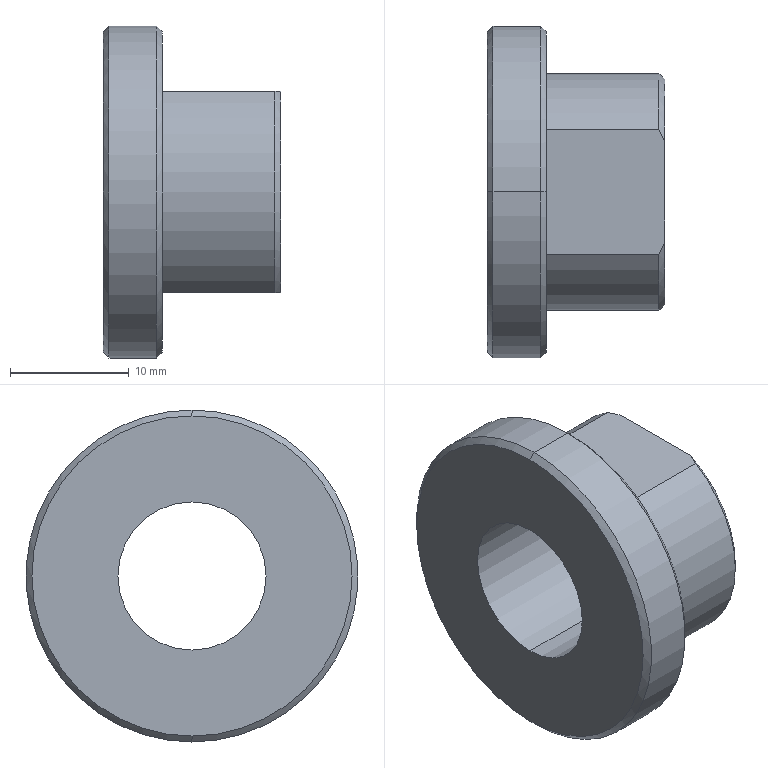Part | SolidWorks | features BaseBody 1 | 1 solid | 17 faces | box 15 x 28 x 28 mm | volume 4139 mm3 | cylinder 6 | cone 6 | plane 5 | commonest cylinder face diameters 12.5 x2 20 x2 28 x2
STEP:
#1=CARTESIAN_POINT('',(0.,0.,6.25));
#2=VERTEX_POINT('',#1);
#3=CARTESIAN_POINT('',(0.,0.,-6.25));
#4=VERTEX_POINT('',#3);
#5=CARTESIAN_POINT('',(0.,0.,0.));
#6=DIRECTION('',(1.,0.,0.));
#7=DIRECTION('',(0.,0.,-1.));
#8=AXIS2_PLACEMENT_3D('',#5,#6,#7);
#9=CIRCLE('',#8,6.25);
#10=EDGE_CURVE('',#2,#4,#9,.T.);
#11=ORIENTED_EDGE('',*,*,#10,.F.);
#12=CARTESIAN_POINT('',(15.,0.,6.25));
#13=VERTEX_POINT('',#12);
#14=CARTESIAN_POINT('',(15.,0.,6.25));
#15=DIRECTION('',(1.,0.,0.));
#16=VECTOR('',#15,1000.);
#17=LINE('',#14,#16);
#18=EDGE_CURVE('',#2,#13,#17,.T.);
#19=ORIENTED_EDGE('',*,*,#18,.T.);
#20=CARTESIAN_POINT('',(15.,0.,-6.25));
#21=VERTEX_POINT('',#20);
#22=CARTESIAN_POINT('',(15.,0.,0.));
#23=DIRECTION('',(1.,0.,0.));
#24=DIRECTION('',(0.,0.,-1.));
#25=AXIS2_PLACEMENT_3D('',#22,#23,#24);
#26=CIRCLE('',#25,6.25);
#27=EDGE_CURVE('',#13,#21,#26,.T.);
#28=ORIENTED_EDGE('',*,*,#27,.T.);
#29=CARTESIAN_POINT('',(15.,0.,-6.25));
#30=DIRECTION('',(1.,0.,0.));
#31=VECTOR('',#30,1000.);
#32=LINE('',#29,#31);
#33=EDGE_CURVE('',#4,#21,#32,.T.);
#34=ORIENTED_EDGE('',*,*,#33,.F.);
#35=EDGE_LOOP('',(#11,#19,#28,#34));
#36=FACE_OUTER_BOUND('',#35,.T.);
#37=CARTESIAN_POINT('',(15.,0.,0.));
#38=DIRECTION('',(1.,0.,0.));
#39=DIRECTION('',(0.,0.,-1.));
#40=AXIS2_PLACEMENT_3D('',#37,#38,#39);
#41=CYLINDRICAL_SURFACE('',#40,6.25);
#42=ADVANCED_FACE('',(#36),#41,.F.);
#43=CARTESIAN_POINT('',(0.,0.,13.5));
#44=VERTEX_POINT('',#43);
#45=CARTESIAN_POINT('',(0.,0.,-13.5));
#46=VERTEX_POINT('',#45);
#47=CARTESIAN_POINT('',(0.,0.,0.));
#48=DIRECTION('',(-1.,0.,0.));
#49=DIRECTION('',(0.,0.,-1.));
#50=AXIS2_PLACEMENT_3D('',#47,#48,#49);
#51=CIRCLE('',#50,13.5);
#52=EDGE_CURVE('',#44,#46,#51,.T.);
#53=ORIENTED_EDGE('',*,*,#52,.F.);
#54=CARTESIAN_POINT('',(0.5,0.,14.));
#55=VERTEX_POINT('',#54);
#56=CARTESIAN_POINT('',(0.5,0.,14.));
#57=DIRECTION('',(0.7071,0.,0.7071));
#58=VECTOR('',#57,1000.);
#59=LINE('',#56,#58);
#60=EDGE_CURVE('',#44,#55,#59,.T.);
#61=ORIENTED_EDGE('',*,*,#60,.T.);
#62=CARTESIAN_POINT('',(0.5,0.,-14.));
#63=VERTEX_POINT('',#62);
#64=CARTESIAN_POINT('',(0.5,0.,0.));
#65=DIRECTION('',(1.,0.,0.));
#66=DIRECTION('',(0.,0.,-1.));
#67=AXIS2_PLACEMENT_3D('',#64,#65,#66);
#68=CIRCLE('',#67,14.);
#69=EDGE_CURVE('',#63,#55,#68,.T.);
#70=ORIENTED_EDGE('',*,*,#69,.F.);
#71=CARTESIAN_POINT('',(0.5,0.,-14.));
#72=DIRECTION('',(0.7071,0.,-0.7071));
#73=VECTOR('',#72,1000.);
#74=LINE('',#71,#73);
#75=EDGE_CURVE('',#46,#63,#74,.T.);
#76=ORIENTED_EDGE('',*,*,#75,.F.);
#77=EDGE_LOOP('',(#53,#61,#70,#76));
#78=FACE_OUTER_BOUND('',#77,.T.);
#79=CARTESIAN_POINT('',(0.5,0.,0.));
#80=DIRECTION('',(1.,0.,0.));
#81=DIRECTION('',(0.,0.,-1.));
#82=AXIS2_PLACEMENT_3D('',#79,#80,#81);
#83=CONICAL_SURFACE('',#82,14.,0.7854);
#84=ADVANCED_FACE('',(#78),#83,.T.);
#85=CARTESIAN_POINT('',(5.,0.,-13.5));
#86=VERTEX_POINT('',#85);
#87=CARTESIAN_POINT('',(5.,0.,13.5));
#88=VERTEX_POINT('',#87);
#89=CARTESIAN_POINT('',(5.,0.,0.));
#90=DIRECTION('',(1.,0.,0.));
#91=DIRECTION('',(0.,0.,-1.));
#92=AXIS2_PLACEMENT_3D('',#89,#90,#91);
#93=CIRCLE('',#92,13.5);
#94=EDGE_CURVE('',#86,#88,#93,.T.);
#95=ORIENTED_EDGE('',*,*,#94,.F.);
#96=CARTESIAN_POINT('',(4.5,0.,-14.));
#97=VERTEX_POINT('',#96);
#98=CARTESIAN_POINT('',(5.,0.,-13.5));
#99=DIRECTION('',(-0.7071,0.,-0.7071));
#100=VECTOR('',#99,1000.);
#101=LINE('',#98,#100);
#102=EDGE_CURVE('',#86,#97,#101,.T.);
#103=ORIENTED_EDGE('',*,*,#102,.T.);
#104=CARTESIAN_POINT('',(4.5,0.,14.));
#105=VERTEX_POINT('',#104);
#106=CARTESIAN_POINT('',(4.5,0.,0.));
#107=DIRECTION('',(-1.,0.,0.));
#108=DIRECTION('',(0.,0.,-1.));
#109=AXIS2_PLACEMENT_3D('',#106,#107,#108);
#110=CIRCLE('',#109,14.);
#111=EDGE_CURVE('',#105,#97,#110,.T.);
#112=ORIENTED_EDGE('',*,*,#111,.F.);
#113=CARTESIAN_POINT('',(5.,0.,13.5));
#114=DIRECTION('',(-0.7071,0.,0.7071));
#115=VECTOR('',#114,1000.);
#116=LINE('',#113,#115);
#117=EDGE_CURVE('',#88,#105,#116,.T.);
#118=ORIENTED_EDGE('',*,*,#117,.F.);
#119=EDGE_LOOP('',(#95,#103,#112,#118));
#120=FACE_OUTER_BOUND('',#119,.T.);
#121=CARTESIAN_POINT('',(5.,0.,0.));
#122=DIRECTION('',(-1.,0.,0.));
#123=DIRECTION('',(0.,0.,1.));
#124=AXIS2_PLACEMENT_3D('',#121,#122,#123);
#125=CONICAL_SURFACE('',#124,13.5,0.7854);
#126=ADVANCED_FACE('',(#120),#125,.T.);
#127=ORIENTED_EDGE('',*,*,#111,.T.);
#128=CARTESIAN_POINT('',(5.,0.,-14.));
#129=DIRECTION('',(-1.,0.,0.));
#130=VECTOR('',#129,1000.);
#131=LINE('',#128,#130);
#132=EDGE_CURVE('',#97,#63,#131,.T.);
#133=ORIENTED_EDGE('',*,*,#132,.T.);
#134=ORIENTED_EDGE('',*,*,#69,.T.);
#135=CARTESIAN_POINT('',(5.,0.,14.));
#136=DIRECTION('',(-1.,0.,0.));
#137=VECTOR('',#136,1000.);
#138=LINE('',#135,#137);
#139=EDGE_CURVE('',#105,#55,#138,.T.);
#140=ORIENTED_EDGE('',*,*,#139,.F.);
#141=EDGE_LOOP('',(#127,#133,#134,#140));
#142=FACE_OUTER_BOUND('',#141,.T.);
#143=CARTESIAN_POINT('',(5.,0.,0.));
#144=DIRECTION('',(-1.,0.,0.));
#145=DIRECTION('',(0.,0.,1.));
#146=AXIS2_PLACEMENT_3D('',#143,#144,#145);
#147=CYLINDRICAL_SURFACE('',#146,14.);
#148=ADVANCED_FACE('',(#142),#147,.T.);
#149=CARTESIAN_POINT('',(14.5,-5.268,-8.5));
#150=VERTEX_POINT('',#149);
#151=CARTESIAN_POINT('',(14.5,-5.268,8.5));
#152=VERTEX_POINT('',#151);
#153=CARTESIAN_POINT('',(14.5,0.,0.));
#154=DIRECTION('',(-1.,0.,0.));
#155=DIRECTION('',(0.,0.,-1.));
#156=AXIS2_PLACEMENT_3D('',#153,#154,#155);
#157=CIRCLE('',#156,10.);
#158=EDGE_CURVE('',#150,#152,#157,.T.);
#159=ORIENTED_EDGE('',*,*,#158,.T.);
#160=CARTESIAN_POINT('',(5.,-5.268,8.5));
#161=VERTEX_POINT('',#160);
#162=CARTESIAN_POINT('',(15.,-5.268,8.5));
#163=DIRECTION('',(-1.,0.,0.));
#164=VECTOR('',#163,1000.);
#165=LINE('',#162,#164);
#166=EDGE_CURVE('',#152,#161,#165,.T.);
#167=ORIENTED_EDGE('',*,*,#166,.T.);
#168=CARTESIAN_POINT('',(5.,-5.268,-8.5));
#169=VERTEX_POINT('',#168);
#170=CARTESIAN_POINT('',(5.,0.,0.));
#171=DIRECTION('',(1.,0.,0.));
#172=DIRECTION('',(0.,0.,-1.));
#173=AXIS2_PLACEMENT_3D('',#170,#171,#172);
#174=CIRCLE('',#173,10.);
#175=EDGE_CURVE('',#161,#169,#174,.T.);
#176=ORIENTED_EDGE('',*,*,#175,.T.);
#177=CARTESIAN_POINT('',(15.,-5.268,-8.5));
#178=DIRECTION('',(1.,0.,0.));
#179=VECTOR('',#178,1000.);
#180=LINE('',#177,#179);
#181=EDGE_CURVE('',#169,#150,#180,.T.);
#182=ORIENTED_EDGE('',*,*,#181,.T.);
#183=EDGE_LOOP('',(#159,#167,#176,#182));
#184=FACE_OUTER_BOUND('',#183,.T.);
#185=CARTESIAN_POINT('',(15.,0.,0.));
#186=DIRECTION('',(-1.,0.,0.));
#187=DIRECTION('',(0.,0.,1.));
#188=AXIS2_PLACEMENT_3D('',#185,#186,#187);
#189=CYLINDRICAL_SURFACE('',#188,10.);
#190=ADVANCED_FACE('',(#184),#189,.T.);
#191=CARTESIAN_POINT('',(15.,-4.243,8.5));
#192=VERTEX_POINT('',#191);
#193=CARTESIAN_POINT('',(14.5,-5.268,8.5));
#194=CARTESIAN_POINT('',(14.677,-4.931,8.5));
#195=CARTESIAN_POINT('',(14.845,-4.59,8.5));
#196=CARTESIAN_POINT('',(15.,-4.243,8.5));
#197=B_SPLINE_CURVE_WITH_KNOTS('',3,(#193,#194,#195,#196),.UNSPECIFIED.,.F.,.F.,(4,4),(0.01928,0.02042),.UNSPECIFIED.);
#198=EDGE_CURVE('',#152,#192,#197,.T.);
#199=ORIENTED_EDGE('',*,*,#198,.F.);
#200=ORIENTED_EDGE('',*,*,#158,.F.);
#201=CARTESIAN_POINT('',(15.,-4.243,-8.5));
#202=VERTEX_POINT('',#201);
#203=CARTESIAN_POINT('',(15.,-4.243,-8.5));
#204=CARTESIAN_POINT('',(14.844,-4.591,-8.5));
#205=CARTESIAN_POINT('',(14.677,-4.932,-8.5));
#206=CARTESIAN_POINT('',(14.5,-5.268,-8.5));
#207=B_SPLINE_CURVE_WITH_KNOTS('',3,(#203,#204,#205,#206),.UNSPECIFIED.,.F.,.F.,(4,4),(0.02921,0.03036),.UNSPECIFIED.);
#208=EDGE_CURVE('',#202,#150,#207,.T.);
#209=ORIENTED_EDGE('',*,*,#208,.F.);
#210=CARTESIAN_POINT('',(15.,0.,0.));
#211=DIRECTION('',(1.,0.,0.));
#212=DIRECTION('',(0.,0.,-1.));
#213=AXIS2_PLACEMENT_3D('',#210,#211,#212);
#214=CIRCLE('',#213,9.5);
#215=EDGE_CURVE('',#192,#202,#214,.T.);
#216=ORIENTED_EDGE('',*,*,#215,.F.);
#217=EDGE_LOOP('',(#199,#200,#209,#216));
#218=FACE_OUTER_BOUND('',#217,.T.);
#219=CARTESIAN_POINT('',(15.,0.,0.));
#220=DIRECTION('',(-1.,0.,0.));
#221=DIRECTION('',(0.,0.,1.));
#222=AXIS2_PLACEMENT_3D('',#219,#220,#221);
#223=CONICAL_SURFACE('',#222,9.5,0.7854);
#224=ADVANCED_FACE('',(#218),#223,.T.);
#225=CARTESIAN_POINT('',(5.,0.,0.));
#226=DIRECTION('',(1.,0.,0.));
#227=DIRECTION('',(0.,0.,-1.));
#228=AXIS2_PLACEMENT_3D('',#225,#226,#227);
#229=CIRCLE('',#228,13.5);
#230=EDGE_CURVE('',#88,#86,#229,.T.);
#231=ORIENTED_EDGE('',*,*,#230,.T.);
#232=ORIENTED_EDGE('',*,*,#94,.T.);
#233=EDGE_LOOP('',(#231,#232));
#234=FACE_OUTER_BOUND('',#233,.T.);
#235=ORIENTED_EDGE('',*,*,#175,.F.);
#236=CARTESIAN_POINT('',(5.,5.268,8.5));
#237=VERTEX_POINT('',#236);
#238=CARTESIAN_POINT('',(5.,-10.,8.5));
#239=DIRECTION('',(0.,1.,0.));
#240=VECTOR('',#239,1000.);
#241=LINE('',#238,#240);
#242=EDGE_CURVE('',#161,#237,#241,.T.);
#243=ORIENTED_EDGE('',*,*,#242,.T.);
#244=CARTESIAN_POINT('',(5.,5.268,-8.5));
#245=VERTEX_POINT('',#244);
#246=CARTESIAN_POINT('',(5.,0.,0.));
#247=DIRECTION('',(1.,0.,0.));
#248=DIRECTION('',(0.,0.,-1.));
#249=AXIS2_PLACEMENT_3D('',#246,#247,#248);
#250=CIRCLE('',#249,10.);
#251=EDGE_CURVE('',#245,#237,#250,.T.);
#252=ORIENTED_EDGE('',*,*,#251,.F.);
#253=CARTESIAN_POINT('',(5.,-10.,-8.5));
#254=DIRECTION('',(0.,-1.,0.));
#255=VECTOR('',#254,1000.);
#256=LINE('',#253,#255);
#257=EDGE_CURVE('',#245,#169,#256,.T.);
#258=ORIENTED_EDGE('',*,*,#257,.T.);
#259=EDGE_LOOP('',(#235,#243,#252,#258));
#260=FACE_BOUND('',#259,.T.);
#261=CARTESIAN_POINT('',(5.,0.,0.));
#262=DIRECTION('',(1.,0.,0.));
#263=DIRECTION('',(0.,0.,-1.));
#264=AXIS2_PLACEMENT_3D('',#261,#262,#263);
#265=PLANE('',#264);
#266=ADVANCED_FACE('',(#234,#260),#265,.T.);
#267=ORIENTED_EDGE('',*,*,#132,.F.);
#268=CARTESIAN_POINT('',(4.5,0.,0.));
#269=DIRECTION('',(-1.,0.,0.));
#270=DIRECTION('',(0.,0.,-1.));
#271=AXIS2_PLACEMENT_3D('',#268,#269,#270);
#272=CIRCLE('',#271,14.);
#273=EDGE_CURVE('',#97,#105,#272,.T.);
#274=ORIENTED_EDGE('',*,*,#273,.T.);
#275=ORIENTED_EDGE('',*,*,#139,.T.);
#276=CARTESIAN_POINT('',(0.5,0.,0.));
#277=DIRECTION('',(1.,0.,0.));
#278=DIRECTION('',(0.,0.,-1.));
#279=AXIS2_PLACEMENT_3D('',#276,#277,#278);
#280=CIRCLE('',#279,14.);
#281=EDGE_CURVE('',#55,#63,#280,.T.);
#282=ORIENTED_EDGE('',*,*,#281,.T.);
#283=EDGE_LOOP('',(#267,#274,#275,#282));
#284=FACE_OUTER_BOUND('',#283,.T.);
#285=CARTESIAN_POINT('',(5.,0.,0.));
#286=DIRECTION('',(-1.,0.,0.));
#287=DIRECTION('',(0.,0.,1.));
#288=AXIS2_PLACEMENT_3D('',#285,#286,#287);
#289=CYLINDRICAL_SURFACE('',#288,14.);
#290=ADVANCED_FACE('',(#284),#289,.T.);
#291=CARTESIAN_POINT('',(0.,0.,0.));
#292=DIRECTION('',(1.,0.,0.));
#293=DIRECTION('',(0.,0.,-1.));
#294=AXIS2_PLACEMENT_3D('',#291,#292,#293);
#295=CIRCLE('',#294,6.25);
#296=EDGE_CURVE('',#4,#2,#295,.T.);
#297=ORIENTED_EDGE('',*,*,#296,.T.);
#298=ORIENTED_EDGE('',*,*,#10,.T.);
#299=EDGE_LOOP('',(#297,#298));
#300=FACE_BOUND('',#299,.T.);
#301=CARTESIAN_POINT('',(0.,0.,0.));
#302=DIRECTION('',(-1.,0.,0.));
#303=DIRECTION('',(0.,0.,-1.));
#304=AXIS2_PLACEMENT_3D('',#301,#302,#303);
#305=CIRCLE('',#304,13.5);
#306=EDGE_CURVE('',#46,#44,#305,.T.);
#307=ORIENTED_EDGE('',*,*,#306,.T.);
#308=ORIENTED_EDGE('',*,*,#52,.T.);
#309=EDGE_LOOP('',(#307,#308));
#310=FACE_OUTER_BOUND('',#309,.T.);
#311=CARTESIAN_POINT('',(0.,0.,0.));
#312=DIRECTION('',(1.,0.,0.));
#313=DIRECTION('',(0.,0.,-1.));
#314=AXIS2_PLACEMENT_3D('',#311,#312,#313);
#315=PLANE('',#314);
#316=ADVANCED_FACE('',(#300,#310),#315,.F.);
#317=ORIENTED_EDGE('',*,*,#251,.T.);
#318=CARTESIAN_POINT('',(14.5,5.268,8.5));
#319=VERTEX_POINT('',#318);
#320=CARTESIAN_POINT('',(15.,5.268,8.5));
#321=DIRECTION('',(1.,0.,0.));
#322=VECTOR('',#321,1000.);
#323=LINE('',#320,#322);
#324=EDGE_CURVE('',#237,#319,#323,.T.);
#325=ORIENTED_EDGE('',*,*,#324,.T.);
#326=CARTESIAN_POINT('',(14.5,5.268,-8.5));
#327=VERTEX_POINT('',#326);
#328=CARTESIAN_POINT('',(14.5,0.,0.));
#329=DIRECTION('',(-1.,0.,0.));
#330=DIRECTION('',(0.,0.,-1.));
#331=AXIS2_PLACEMENT_3D('',#328,#329,#330);
#332=CIRCLE('',#331,10.);
#333=EDGE_CURVE('',#319,#327,#332,.T.);
#334=ORIENTED_EDGE('',*,*,#333,.T.);
#335=CARTESIAN_POINT('',(15.,5.268,-8.5));
#336=DIRECTION('',(-1.,0.,0.));
#337=VECTOR('',#336,1000.);
#338=LINE('',#335,#337);
#339=EDGE_CURVE('',#327,#245,#338,.T.);
#340=ORIENTED_EDGE('',*,*,#339,.T.);
#341=EDGE_LOOP('',(#317,#325,#334,#340));
#342=FACE_OUTER_BOUND('',#341,.T.);
#343=CARTESIAN_POINT('',(15.,0.,0.));
#344=DIRECTION('',(-1.,0.,0.));
#345=DIRECTION('',(0.,0.,1.));
#346=AXIS2_PLACEMENT_3D('',#343,#344,#345);
#347=CYLINDRICAL_SURFACE('',#346,10.);
#348=ADVANCED_FACE('',(#342),#347,.T.);
#349=CARTESIAN_POINT('',(15.,4.243,8.5));
#350=VERTEX_POINT('',#349);
#351=CARTESIAN_POINT('',(15.,-10.,8.5));
#352=DIRECTION('',(0.,1.,0.));
#353=VECTOR('',#352,1000.);
#354=LINE('',#351,#353);
#355=EDGE_CURVE('',#192,#350,#354,.T.);
#356=ORIENTED_EDGE('',*,*,#355,.F.);
#357=ORIENTED_EDGE('',*,*,#215,.T.);
#358=CARTESIAN_POINT('',(15.,4.243,-8.5));
#359=VERTEX_POINT('',#358);
#360=CARTESIAN_POINT('',(15.,-10.,-8.5));
#361=DIRECTION('',(0.,-1.,0.));
#362=VECTOR('',#361,1000.);
#363=LINE('',#360,#362);
#364=EDGE_CURVE('',#359,#202,#363,.T.);
#365=ORIENTED_EDGE('',*,*,#364,.F.);
#366=CARTESIAN_POINT('',(15.,0.,0.));
#367=DIRECTION('',(1.,0.,0.));
#368=DIRECTION('',(0.,0.,-1.));
#369=AXIS2_PLACEMENT_3D('',#366,#367,#368);
#370=CIRCLE('',#369,9.5);
#371=EDGE_CURVE('',#359,#350,#370,.T.);
#372=ORIENTED_EDGE('',*,*,#371,.T.);
#373=EDGE_LOOP('',(#356,#357,#365,#372));
#374=FACE_OUTER_BOUND('',#373,.T.);
#375=CARTESIAN_POINT('',(15.,0.,0.));
#376=DIRECTION('',(1.,0.,0.));
#377=DIRECTION('',(0.,0.,-1.));
#378=AXIS2_PLACEMENT_3D('',#375,#376,#377);
#379=CIRCLE('',#378,6.25);
#380=EDGE_CURVE('',#21,#13,#379,.T.);
#381=ORIENTED_EDGE('',*,*,#380,.F.);
#382=ORIENTED_EDGE('',*,*,#27,.F.);
#383=EDGE_LOOP('',(#381,#382));
#384=FACE_BOUND('',#383,.T.);
#385=CARTESIAN_POINT('',(15.,0.,0.));
#386=DIRECTION('',(1.,0.,0.));
#387=DIRECTION('',(0.,0.,-1.));
#388=AXIS2_PLACEMENT_3D('',#385,#386,#387);
#389=PLANE('',#388);
#390=ADVANCED_FACE('',(#374,#384),#389,.T.);
#391=ORIENTED_EDGE('',*,*,#102,.F.);
#392=ORIENTED_EDGE('',*,*,#230,.F.);
#393=ORIENTED_EDGE('',*,*,#117,.T.);
#394=ORIENTED_EDGE('',*,*,#273,.F.);
#395=EDGE_LOOP('',(#391,#392,#393,#394));
#396=FACE_OUTER_BOUND('',#395,.T.);
#397=CARTESIAN_POINT('',(5.,0.,0.));
#398=DIRECTION('',(-1.,0.,0.));
#399=DIRECTION('',(0.,0.,1.));
#400=AXIS2_PLACEMENT_3D('',#397,#398,#399);
#401=CONICAL_SURFACE('',#400,13.5,0.7854);
#402=ADVANCED_FACE('',(#396),#401,.T.);
#403=CARTESIAN_POINT('',(15.,4.243,8.5));
#404=CARTESIAN_POINT('',(14.844,4.591,8.5));
#405=CARTESIAN_POINT('',(14.677,4.932,8.5));
#406=CARTESIAN_POINT('',(14.5,5.268,8.5));
#407=B_SPLINE_CURVE_WITH_KNOTS('',3,(#403,#404,#405,#406),.UNSPECIFIED.,.F.,.F.,(4,4),(0.02921,0.03036),.UNSPECIFIED.);
#408=EDGE_CURVE('',#350,#319,#407,.T.);
#409=ORIENTED_EDGE('',*,*,#408,.F.);
#410=ORIENTED_EDGE('',*,*,#371,.F.);
#411=CARTESIAN_POINT('',(14.5,5.268,-8.5));
#412=CARTESIAN_POINT('',(14.677,4.931,-8.5));
#413=CARTESIAN_POINT('',(14.845,4.59,-8.5));
#414=CARTESIAN_POINT('',(15.,4.243,-8.5));
#415=B_SPLINE_CURVE_WITH_KNOTS('',3,(#411,#412,#413,#414),.UNSPECIFIED.,.F.,.F.,(4,4),(0.01928,0.02042),.UNSPECIFIED.);
#416=EDGE_CURVE('',#327,#359,#415,.T.);
#417=ORIENTED_EDGE('',*,*,#416,.F.);
#418=ORIENTED_EDGE('',*,*,#333,.F.);
#419=EDGE_LOOP('',(#409,#410,#417,#418));
#420=FACE_OUTER_BOUND('',#419,.T.);
#421=CARTESIAN_POINT('',(15.,0.,0.));
#422=DIRECTION('',(-1.,0.,0.));
#423=DIRECTION('',(0.,0.,1.));
#424=AXIS2_PLACEMENT_3D('',#421,#422,#423);
#425=CONICAL_SURFACE('',#424,9.5,0.7854);
#426=ADVANCED_FACE('',(#420),#425,.T.);
#427=ORIENTED_EDGE('',*,*,#60,.F.);
#428=ORIENTED_EDGE('',*,*,#306,.F.);
#429=ORIENTED_EDGE('',*,*,#75,.T.);
#430=ORIENTED_EDGE('',*,*,#281,.F.);
#431=EDGE_LOOP('',(#427,#428,#429,#430));
#432=FACE_OUTER_BOUND('',#431,.T.);
#433=CARTESIAN_POINT('',(0.5,0.,0.));
#434=DIRECTION('',(1.,0.,0.));
#435=DIRECTION('',(0.,0.,-1.));
#436=AXIS2_PLACEMENT_3D('',#433,#434,#435);
#437=CONICAL_SURFACE('',#436,14.,0.7854);
#438=ADVANCED_FACE('',(#432),#437,.T.);
#439=ORIENTED_EDGE('',*,*,#18,.F.);
#440=ORIENTED_EDGE('',*,*,#296,.F.);
#441=ORIENTED_EDGE('',*,*,#33,.T.);
#442=ORIENTED_EDGE('',*,*,#380,.T.);
#443=EDGE_LOOP('',(#439,#440,#441,#442));
#444=FACE_OUTER_BOUND('',#443,.T.);
#445=CARTESIAN_POINT('',(15.,0.,0.));
#446=DIRECTION('',(1.,0.,0.));
#447=DIRECTION('',(0.,0.,-1.));
#448=AXIS2_PLACEMENT_3D('',#445,#446,#447);
#449=CYLINDRICAL_SURFACE('',#448,6.25);
#450=ADVANCED_FACE('',(#444),#449,.F.);
#451=ORIENTED_EDGE('',*,*,#416,.T.);
#452=ORIENTED_EDGE('',*,*,#364,.T.);
#453=ORIENTED_EDGE('',*,*,#208,.T.);
#454=ORIENTED_EDGE('',*,*,#181,.F.);
#455=ORIENTED_EDGE('',*,*,#257,.F.);
#456=ORIENTED_EDGE('',*,*,#339,.F.);
#457=EDGE_LOOP('',(#451,#452,#453,#454,#455,#456));
#458=FACE_OUTER_BOUND('',#457,.T.);
#459=CARTESIAN_POINT('',(5.,-10.,-8.5));
#460=DIRECTION('',(0.,0.,1.));
#461=DIRECTION('',(1.,0.,0.));
#462=AXIS2_PLACEMENT_3D('',#459,#460,#461);
#463=PLANE('',#462);
#464=ADVANCED_FACE('',(#458),#463,.F.);
#465=ORIENTED_EDGE('',*,*,#198,.T.);
#466=ORIENTED_EDGE('',*,*,#355,.T.);
#467=ORIENTED_EDGE('',*,*,#408,.T.);
#468=ORIENTED_EDGE('',*,*,#324,.F.);
#469=ORIENTED_EDGE('',*,*,#242,.F.);
#470=ORIENTED_EDGE('',*,*,#166,.F.);
#471=EDGE_LOOP('',(#465,#466,#467,#468,#469,#470));
#472=FACE_OUTER_BOUND('',#471,.T.);
#473=CARTESIAN_POINT('',(5.,-10.,8.5));
#474=DIRECTION('',(0.,0.,-1.));
#475=DIRECTION('',(-1.,0.,0.));
#476=AXIS2_PLACEMENT_3D('',#473,#474,#475);
#477=PLANE('',#476);
#478=ADVANCED_FACE('',(#472),#477,.F.);
#479=CLOSED_SHELL('',(#42,#84,#126,#148,#190,#224,#266,#290,#316,#348,#390,#402,#426,#438,#450,#464,#478));
#480=MANIFOLD_SOLID_BREP('',#479);
#481=CARTESIAN_POINT('',(0.,0.,0.));
#482=DIRECTION('',(0.,0.,1.));
#483=DIRECTION('',(1.,0.,0.));
#484=AXIS2_PLACEMENT_3D('',#481,#482,#483);
#485=(LENGTH_UNIT()NAMED_UNIT(*)SI_UNIT(.MILLI.,.METRE.));
#486=UNCERTAINTY_MEASURE_WITH_UNIT(LENGTH_MEASURE(0.00001),#485,'','');
#487=(NAMED_UNIT(*)PLANE_ANGLE_UNIT()SI_UNIT($,.RADIAN.));
#488=(NAMED_UNIT(*)SI_UNIT($,.STERADIAN.)SOLID_ANGLE_UNIT());
#489=(GEOMETRIC_REPRESENTATION_CONTEXT(3)GLOBAL_UNCERTAINTY_ASSIGNED_CONTEXT((#486))GLOBAL_UNIT_ASSIGNED_CONTEXT((#485,#487,#488))REPRESENTATION_CONTEXT('',''));
#490=ADVANCED_BREP_SHAPE_REPRESENTATION('',(#480,#484),#489);